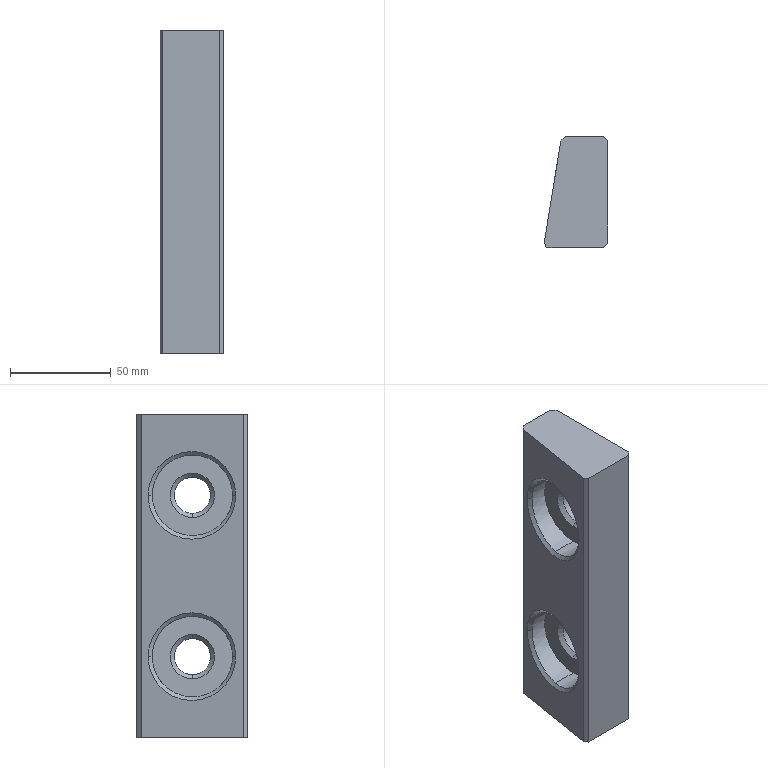Part | SolidWorks | features Chamfer 2, ICE 2, Extrusion 1 | 1 solid | 28 faces | box 31.677 x 55 x 160 mm | volume 198340 mm3 | plane 12 | cylinder 8 | spline 4 | cone 4 | commonest cylinder face diameters 18 x4 40 x4